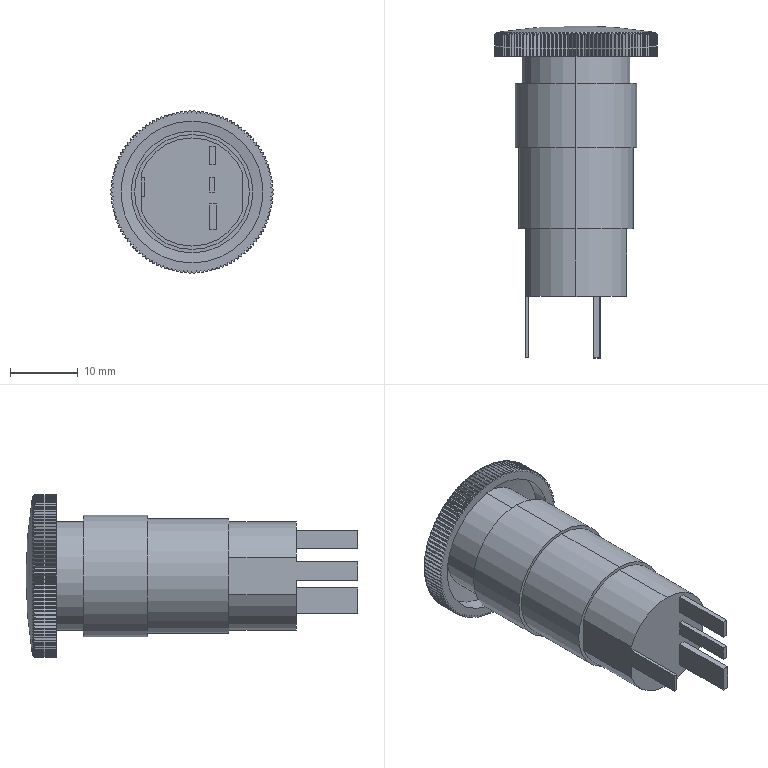Part | STEP file | emergency stop button LAS1-AY-22TS-R | 1 solid | 401 faces | box 23.995 x 49.1 x 23.995 mm | volume 9425 mm3 | plane 266 | cylinder 131 | torus 2 | sphere 2 | commonest cylinder face diameters 24 x120 16 x5 17 x2 18 x2 21 x2